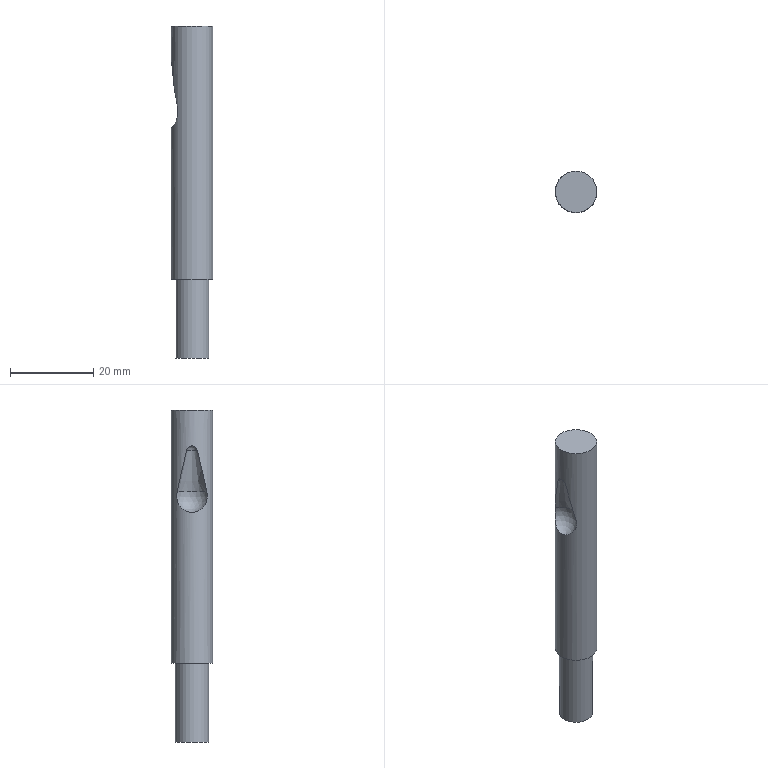Part | NX | features solid 2 | 1 solid | 8 faces | volume 5568 mm3 | plane 3 | cylinder 2 | sphere 2 | cone 1 | commonest cylinder face diameters 8 x1 10 x1